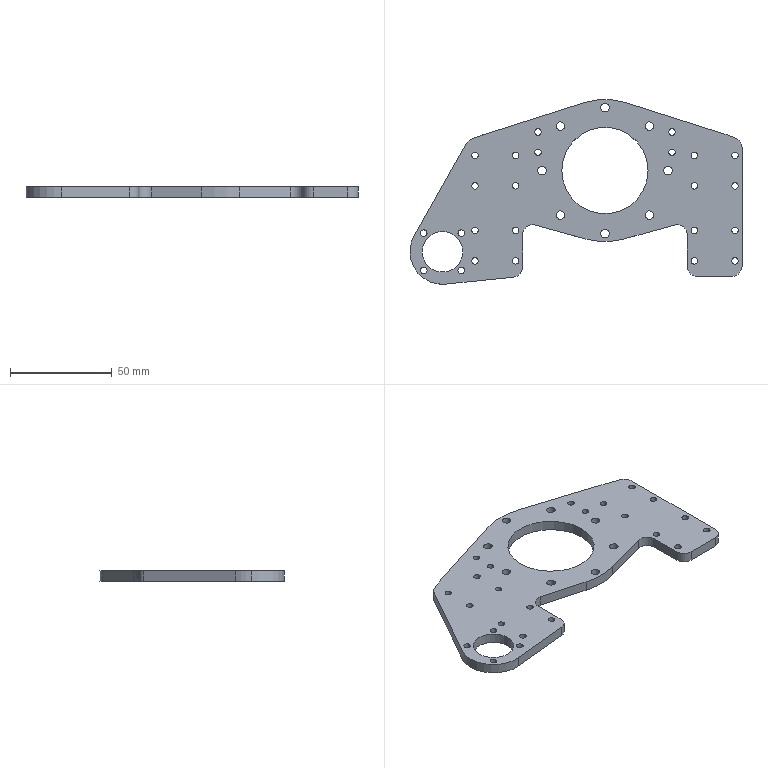Part | SolidWorks | features ICE 10, Fillet 5, MirrorPattern 2, Extrusion 1 | 1 solid | 93 faces | box 163.5 x 91 x 5 mm | volume 40085 mm3 | cylinder 79 | plane 12 | spline 2 | commonest cylinder face diameters 3.2 x48 4.2 x16 10 x7 20 x2 32 x2 42.5 x2